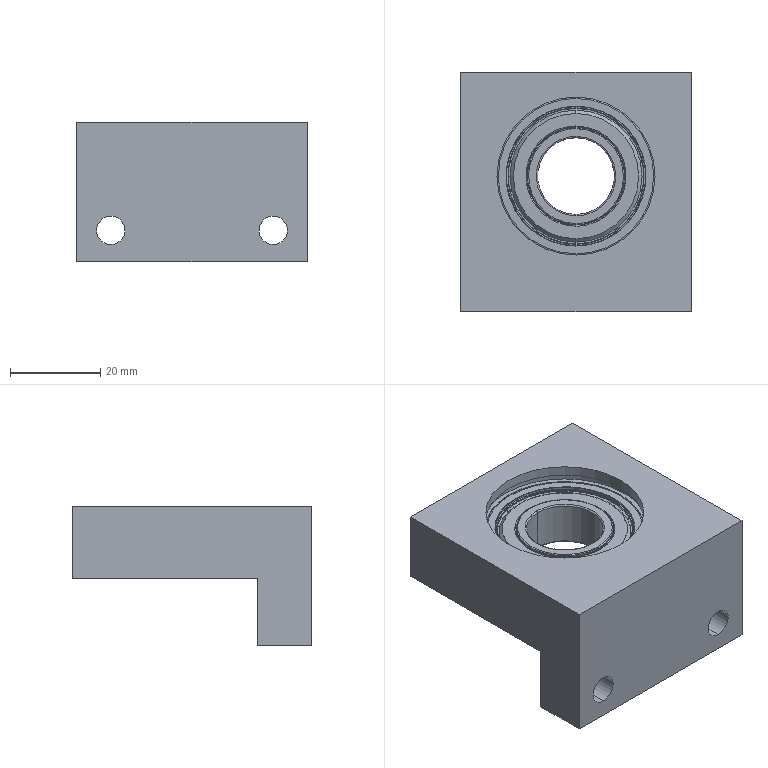Part | SolidWorks | features BaseBody 2 | 2 solids | 159 faces | box 51 x 53 x 31 mm | volume 42368 mm3 | spline 52 | cylinder 44 | cone 40 | plane 23 | commonest cylinder face diameters 35 x6 6.3 x4 20.6 x4 21.4 x4 21.8 x4 22.2 x4